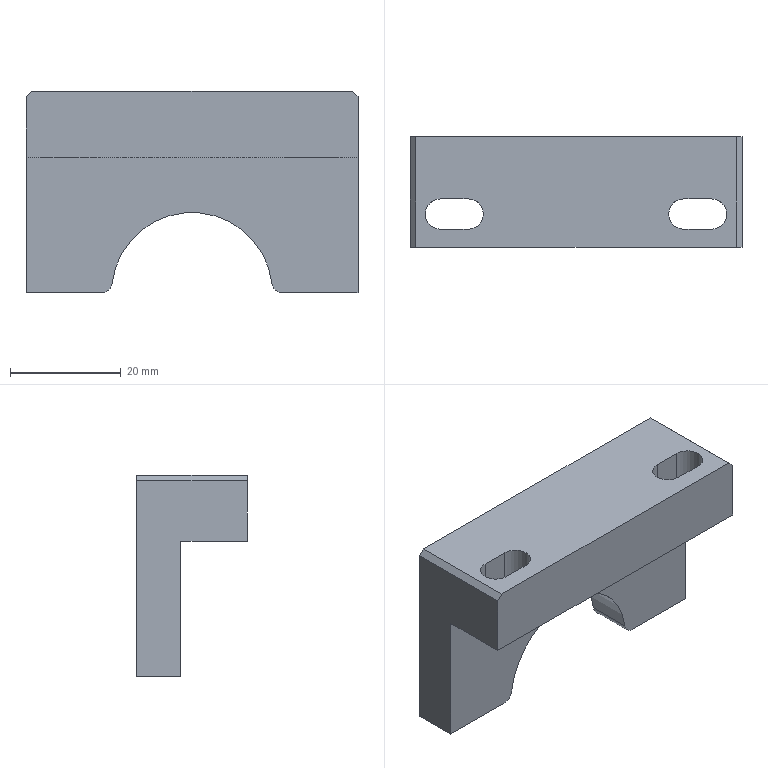Part | NX | 1 solid | 26 faces | box 60 x 20 x 36.5 mm | volume 22060 mm3 | plane 15 | cylinder 9 | cone 2 | commonest cylinder face diameters 5.5 x4 3.3 x2 4 x2 29.1 x1
STEP:
#1=CARTESIAN_POINT('',(24.5,3.75,6.25));
#2=VERTEX_POINT('',#1);
#3=CARTESIAN_POINT('',(24.5,3.75,18.25));
#4=VERTEX_POINT('',#3);
#5=CARTESIAN_POINT('',(24.5,3.75,-18.25));
#6=DIRECTION('',(0.,0.,1.));
#7=VECTOR('',#6,1000.);
#8=LINE('',#5,#7);
#9=EDGE_CURVE('',#2,#4,#8,.T.);
#10=ORIENTED_EDGE('',*,*,#9,.T.);
#11=CARTESIAN_POINT('',(19.5,3.75,18.25));
#12=VERTEX_POINT('',#11);
#13=CARTESIAN_POINT('',(24.5,3.75,18.25));
#14=DIRECTION('',(-1.,0.,0.));
#15=VECTOR('',#14,1000.);
#16=LINE('',#13,#15);
#17=EDGE_CURVE('',#4,#12,#16,.T.);
#18=ORIENTED_EDGE('',*,*,#17,.T.);
#19=CARTESIAN_POINT('',(19.5,3.75,6.25));
#20=VERTEX_POINT('',#19);
#21=CARTESIAN_POINT('',(19.5,3.75,-18.25));
#22=DIRECTION('',(0.,0.,1.));
#23=VECTOR('',#22,1000.);
#24=LINE('',#21,#23);
#25=EDGE_CURVE('',#20,#12,#24,.T.);
#26=ORIENTED_EDGE('',*,*,#25,.F.);
#27=CARTESIAN_POINT('',(-30.,3.75,6.25));
#28=DIRECTION('',(-1.,0.,0.));
#29=VECTOR('',#28,1000.);
#30=LINE('',#27,#29);
#31=EDGE_CURVE('',#2,#20,#30,.T.);
#32=ORIENTED_EDGE('',*,*,#31,.F.);
#33=EDGE_LOOP('',(#10,#18,#26,#32));
#34=FACE_BOUND('',#33,.T.);
#35=CARTESIAN_POINT('',(24.5,3.75,-18.25));
#36=DIRECTION('',(0.,1.,0.));
#37=DIRECTION('',(-1.,0.,0.));
#38=AXIS2_PLACEMENT_3D('',#35,#36,#37);
#39=PLANE('',#38);
#40=ADVANCED_FACE('',(#34),#39,.F.);
#41=ORIENTED_EDGE('',*,*,#25,.T.);
#42=CARTESIAN_POINT('',(19.5,-1.75,18.25));
#43=VERTEX_POINT('',#42);
#44=CARTESIAN_POINT('',(19.5,1.,18.25));
#45=DIRECTION('',(0.,0.,1.));
#46=DIRECTION('',(1.,0.,0.));
#47=AXIS2_PLACEMENT_3D('',#44,#45,#46);
#48=CIRCLE('',#47,2.75);
#49=EDGE_CURVE('',#12,#43,#48,.T.);
#50=ORIENTED_EDGE('',*,*,#49,.T.);
#51=CARTESIAN_POINT('',(19.5,-1.75,6.25));
#52=VERTEX_POINT('',#51);
#53=CARTESIAN_POINT('',(19.5,-1.75,-18.25));
#54=DIRECTION('',(0.,0.,1.));
#55=VECTOR('',#54,1000.);
#56=LINE('',#53,#55);
#57=EDGE_CURVE('',#52,#43,#56,.T.);
#58=ORIENTED_EDGE('',*,*,#57,.F.);
#59=CARTESIAN_POINT('',(19.5,1.,6.25));
#60=DIRECTION('',(0.,0.,1.));
#61=DIRECTION('',(1.,0.,0.));
#62=AXIS2_PLACEMENT_3D('',#59,#60,#61);
#63=CIRCLE('',#62,2.75);
#64=EDGE_CURVE('',#20,#52,#63,.T.);
#65=ORIENTED_EDGE('',*,*,#64,.F.);
#66=EDGE_LOOP('',(#41,#50,#58,#65));
#67=FACE_BOUND('',#66,.T.);
#68=CARTESIAN_POINT('',(19.5,1.,-18.25));
#69=DIRECTION('',(0.,0.,1.));
#70=DIRECTION('',(1.,0.,0.));
#71=AXIS2_PLACEMENT_3D('',#68,#69,#70);
#72=CYLINDRICAL_SURFACE('',#71,2.75);
#73=ADVANCED_FACE('',(#67),#72,.F.);
#74=ORIENTED_EDGE('',*,*,#57,.T.);
#75=CARTESIAN_POINT('',(24.5,-1.75,18.25));
#76=VERTEX_POINT('',#75);
#77=CARTESIAN_POINT('',(24.5,-1.75,18.25));
#78=DIRECTION('',(1.,0.,0.));
#79=VECTOR('',#78,1000.);
#80=LINE('',#77,#79);
#81=EDGE_CURVE('',#43,#76,#80,.T.);
#82=ORIENTED_EDGE('',*,*,#81,.T.);
#83=CARTESIAN_POINT('',(24.5,-1.75,6.25));
#84=VERTEX_POINT('',#83);
#85=CARTESIAN_POINT('',(24.5,-1.75,-18.25));
#86=DIRECTION('',(0.,0.,1.));
#87=VECTOR('',#86,1000.);
#88=LINE('',#85,#87);
#89=EDGE_CURVE('',#84,#76,#88,.T.);
#90=ORIENTED_EDGE('',*,*,#89,.F.);
#91=CARTESIAN_POINT('',(-30.,-1.75,6.25));
#92=DIRECTION('',(1.,0.,0.));
#93=VECTOR('',#92,1000.);
#94=LINE('',#91,#93);
#95=EDGE_CURVE('',#52,#84,#94,.T.);
#96=ORIENTED_EDGE('',*,*,#95,.F.);
#97=EDGE_LOOP('',(#74,#82,#90,#96));
#98=FACE_BOUND('',#97,.T.);
#99=CARTESIAN_POINT('',(24.5,-1.75,-18.25));
#100=DIRECTION('',(0.,-1.,0.));
#101=DIRECTION('',(1.,0.,0.));
#102=AXIS2_PLACEMENT_3D('',#99,#100,#101);
#103=PLANE('',#102);
#104=ADVANCED_FACE('',(#98),#103,.F.);
#105=CARTESIAN_POINT('',(-19.5,3.75,6.25));
#106=VERTEX_POINT('',#105);
#107=CARTESIAN_POINT('',(-19.5,3.75,18.25));
#108=VERTEX_POINT('',#107);
#109=CARTESIAN_POINT('',(-19.5,3.75,-18.25));
#110=DIRECTION('',(0.,0.,1.));
#111=VECTOR('',#110,1000.);
#112=LINE('',#109,#111);
#113=EDGE_CURVE('',#106,#108,#112,.T.);
#114=ORIENTED_EDGE('',*,*,#113,.T.);
#115=CARTESIAN_POINT('',(-24.5,3.75,18.25));
#116=VERTEX_POINT('',#115);
#117=CARTESIAN_POINT('',(24.5,3.75,18.25));
#118=DIRECTION('',(-1.,0.,0.));
#119=VECTOR('',#118,1000.);
#120=LINE('',#117,#119);
#121=EDGE_CURVE('',#108,#116,#120,.T.);
#122=ORIENTED_EDGE('',*,*,#121,.T.);
#123=CARTESIAN_POINT('',(-24.5,3.75,6.25));
#124=VERTEX_POINT('',#123);
#125=CARTESIAN_POINT('',(-24.5,3.75,-18.25));
#126=DIRECTION('',(0.,0.,1.));
#127=VECTOR('',#126,1000.);
#128=LINE('',#125,#127);
#129=EDGE_CURVE('',#124,#116,#128,.T.);
#130=ORIENTED_EDGE('',*,*,#129,.F.);
#131=CARTESIAN_POINT('',(-30.,3.75,6.25));
#132=DIRECTION('',(-1.,0.,0.));
#133=VECTOR('',#132,1000.);
#134=LINE('',#131,#133);
#135=EDGE_CURVE('',#106,#124,#134,.T.);
#136=ORIENTED_EDGE('',*,*,#135,.F.);
#137=EDGE_LOOP('',(#114,#122,#130,#136));
#138=FACE_BOUND('',#137,.T.);
#139=CARTESIAN_POINT('',(24.5,3.75,-18.25));
#140=DIRECTION('',(0.,1.,0.));
#141=DIRECTION('',(-1.,0.,0.));
#142=AXIS2_PLACEMENT_3D('',#139,#140,#141);
#143=PLANE('',#142);
#144=ADVANCED_FACE('',(#138),#143,.F.);
#145=ORIENTED_EDGE('',*,*,#129,.T.);
#146=CARTESIAN_POINT('',(-24.5,-1.75,18.25));
#147=VERTEX_POINT('',#146);
#148=CARTESIAN_POINT('',(-24.5,1.,18.25));
#149=DIRECTION('',(0.,0.,1.));
#150=DIRECTION('',(1.,0.,0.));
#151=AXIS2_PLACEMENT_3D('',#148,#149,#150);
#152=CIRCLE('',#151,2.75);
#153=EDGE_CURVE('',#116,#147,#152,.T.);
#154=ORIENTED_EDGE('',*,*,#153,.T.);
#155=CARTESIAN_POINT('',(-24.5,-1.75,6.25));
#156=VERTEX_POINT('',#155);
#157=CARTESIAN_POINT('',(-24.5,-1.75,-18.25));
#158=DIRECTION('',(0.,0.,1.));
#159=VECTOR('',#158,1000.);
#160=LINE('',#157,#159);
#161=EDGE_CURVE('',#156,#147,#160,.T.);
#162=ORIENTED_EDGE('',*,*,#161,.F.);
#163=CARTESIAN_POINT('',(-24.5,1.,6.25));
#164=DIRECTION('',(0.,0.,1.));
#165=DIRECTION('',(1.,0.,0.));
#166=AXIS2_PLACEMENT_3D('',#163,#164,#165);
#167=CIRCLE('',#166,2.75);
#168=EDGE_CURVE('',#124,#156,#167,.T.);
#169=ORIENTED_EDGE('',*,*,#168,.F.);
#170=EDGE_LOOP('',(#145,#154,#162,#169));
#171=FACE_BOUND('',#170,.T.);
#172=CARTESIAN_POINT('',(-24.5,1.,-18.25));
#173=DIRECTION('',(0.,0.,1.));
#174=DIRECTION('',(1.,0.,0.));
#175=AXIS2_PLACEMENT_3D('',#172,#173,#174);
#176=CYLINDRICAL_SURFACE('',#175,2.75);
#177=ADVANCED_FACE('',(#171),#176,.F.);
#178=ORIENTED_EDGE('',*,*,#161,.T.);
#179=CARTESIAN_POINT('',(-19.5,-1.75,18.25));
#180=VERTEX_POINT('',#179);
#181=CARTESIAN_POINT('',(24.5,-1.75,18.25));
#182=DIRECTION('',(1.,0.,0.));
#183=VECTOR('',#182,1000.);
#184=LINE('',#181,#183);
#185=EDGE_CURVE('',#147,#180,#184,.T.);
#186=ORIENTED_EDGE('',*,*,#185,.T.);
#187=CARTESIAN_POINT('',(-19.5,-1.75,6.25));
#188=VERTEX_POINT('',#187);
#189=CARTESIAN_POINT('',(-19.5,-1.75,-18.25));
#190=DIRECTION('',(0.,0.,1.));
#191=VECTOR('',#190,1000.);
#192=LINE('',#189,#191);
#193=EDGE_CURVE('',#188,#180,#192,.T.);
#194=ORIENTED_EDGE('',*,*,#193,.F.);
#195=CARTESIAN_POINT('',(-30.,-1.75,6.25));
#196=DIRECTION('',(1.,0.,0.));
#197=VECTOR('',#196,1000.);
#198=LINE('',#195,#197);
#199=EDGE_CURVE('',#156,#188,#198,.T.);
#200=ORIENTED_EDGE('',*,*,#199,.F.);
#201=EDGE_LOOP('',(#178,#186,#194,#200));
#202=FACE_BOUND('',#201,.T.);
#203=CARTESIAN_POINT('',(24.5,-1.75,-18.25));
#204=DIRECTION('',(0.,-1.,0.));
#205=DIRECTION('',(1.,0.,0.));
#206=AXIS2_PLACEMENT_3D('',#203,#204,#205);
#207=PLANE('',#206);
#208=ADVANCED_FACE('',(#202),#207,.F.);
#209=CARTESIAN_POINT('',(14.443,7.,-16.492));
#210=VERTEX_POINT('',#209);
#211=CARTESIAN_POINT('',(16.429,7.,-18.25));
#212=VERTEX_POINT('',#211);
#213=CARTESIAN_POINT('',(16.429,7.,-16.25));
#214=DIRECTION('',(0.,-1.,0.));
#215=DIRECTION('',(0.,0.,1.));
#216=AXIS2_PLACEMENT_3D('',#213,#214,#215);
#217=CIRCLE('',#216,2.);
#218=EDGE_CURVE('',#210,#212,#217,.T.);
#219=ORIENTED_EDGE('',*,*,#218,.T.);
#220=CARTESIAN_POINT('',(30.,7.,-18.25));
#221=VERTEX_POINT('',#220);
#222=CARTESIAN_POINT('',(-30.,7.,-18.25));
#223=DIRECTION('',(1.,0.,0.));
#224=VECTOR('',#223,1000.);
#225=LINE('',#222,#224);
#226=EDGE_CURVE('',#212,#221,#225,.T.);
#227=ORIENTED_EDGE('',*,*,#226,.T.);
#228=CARTESIAN_POINT('',(30.,7.,6.25));
#229=VERTEX_POINT('',#228);
#230=CARTESIAN_POINT('',(30.,7.,-18.25));
#231=DIRECTION('',(0.,0.,1.));
#232=VECTOR('',#231,1000.);
#233=LINE('',#230,#232);
#234=EDGE_CURVE('',#221,#229,#233,.T.);
#235=ORIENTED_EDGE('',*,*,#234,.T.);
#236=CARTESIAN_POINT('',(-30.,7.,6.25));
#237=VERTEX_POINT('',#236);
#238=CARTESIAN_POINT('',(-30.,7.,6.25));
#239=DIRECTION('',(1.,0.,0.));
#240=VECTOR('',#239,1000.);
#241=LINE('',#238,#240);
#242=EDGE_CURVE('',#237,#229,#241,.T.);
#243=ORIENTED_EDGE('',*,*,#242,.F.);
#244=CARTESIAN_POINT('',(-30.,7.,-18.25));
#245=VERTEX_POINT('',#244);
#246=CARTESIAN_POINT('',(-30.,7.,-18.25));
#247=DIRECTION('',(0.,0.,1.));
#248=VECTOR('',#247,1000.);
#249=LINE('',#246,#248);
#250=EDGE_CURVE('',#245,#237,#249,.T.);
#251=ORIENTED_EDGE('',*,*,#250,.F.);
#252=CARTESIAN_POINT('',(-16.429,7.,-18.25));
#253=VERTEX_POINT('',#252);
#254=CARTESIAN_POINT('',(-30.,7.,-18.25));
#255=DIRECTION('',(1.,0.,0.));
#256=VECTOR('',#255,1000.);
#257=LINE('',#254,#256);
#258=EDGE_CURVE('',#245,#253,#257,.T.);
#259=ORIENTED_EDGE('',*,*,#258,.T.);
#260=CARTESIAN_POINT('',(-14.443,7.,-16.492));
#261=VERTEX_POINT('',#260);
#262=CARTESIAN_POINT('',(-16.429,7.,-16.25));
#263=DIRECTION('',(0.,-1.,0.));
#264=DIRECTION('',(0.,0.,1.));
#265=AXIS2_PLACEMENT_3D('',#262,#263,#264);
#266=CIRCLE('',#265,2.);
#267=EDGE_CURVE('',#253,#261,#266,.T.);
#268=ORIENTED_EDGE('',*,*,#267,.T.);
#269=CARTESIAN_POINT('',(0.,7.,-18.25));
#270=DIRECTION('',(0.,-1.,0.));
#271=DIRECTION('',(0.,0.,1.));
#272=AXIS2_PLACEMENT_3D('',#269,#270,#271);
#273=CIRCLE('',#272,14.55);
#274=EDGE_CURVE('',#210,#261,#273,.T.);
#275=ORIENTED_EDGE('',*,*,#274,.F.);
#276=EDGE_LOOP('',(#219,#227,#235,#243,#251,#259,#268,#275));
#277=FACE_BOUND('',#276,.T.);
#278=CARTESIAN_POINT('',(-30.,7.,-18.25));
#279=DIRECTION('',(0.,1.,0.));
#280=DIRECTION('',(0.,0.,1.));
#281=AXIS2_PLACEMENT_3D('',#278,#279,#280);
#282=PLANE('',#281);
#283=ADVANCED_FACE('',(#277),#282,.F.);
#284=CARTESIAN_POINT('',(30.,-5.,6.25));
#285=VERTEX_POINT('',#284);
#286=CARTESIAN_POINT('',(30.,-5.,6.25));
#287=DIRECTION('',(0.,-1.,0.));
#288=VECTOR('',#287,1000.);
#289=LINE('',#286,#288);
#290=EDGE_CURVE('',#229,#285,#289,.T.);
#291=ORIENTED_EDGE('',*,*,#290,.T.);
#292=CARTESIAN_POINT('',(-30.,-5.,6.25));
#293=VERTEX_POINT('',#292);
#294=CARTESIAN_POINT('',(-30.,-5.,6.25));
#295=DIRECTION('',(1.,0.,0.));
#296=VECTOR('',#295,1000.);
#297=LINE('',#294,#296);
#298=EDGE_CURVE('',#293,#285,#297,.T.);
#299=ORIENTED_EDGE('',*,*,#298,.F.);
#300=CARTESIAN_POINT('',(-30.,-5.,6.25));
#301=DIRECTION('',(0.,-1.,0.));
#302=VECTOR('',#301,1000.);
#303=LINE('',#300,#302);
#304=EDGE_CURVE('',#237,#293,#303,.T.);
#305=ORIENTED_EDGE('',*,*,#304,.F.);
#306=ORIENTED_EDGE('',*,*,#242,.T.);
#307=EDGE_LOOP('',(#291,#299,#305,#306));
#308=FACE_BOUND('',#307,.T.);
#309=ORIENTED_EDGE('',*,*,#199,.T.);
#310=CARTESIAN_POINT('',(-19.5,1.,6.25));
#311=DIRECTION('',(0.,0.,1.));
#312=DIRECTION('',(1.,0.,0.));
#313=AXIS2_PLACEMENT_3D('',#310,#311,#312);
#314=CIRCLE('',#313,2.75);
#315=EDGE_CURVE('',#188,#106,#314,.T.);
#316=ORIENTED_EDGE('',*,*,#315,.T.);
#317=ORIENTED_EDGE('',*,*,#135,.T.);
#318=ORIENTED_EDGE('',*,*,#168,.T.);
#319=EDGE_LOOP('',(#309,#316,#317,#318));
#320=FACE_BOUND('',#319,.T.);
#321=ORIENTED_EDGE('',*,*,#95,.T.);
#322=CARTESIAN_POINT('',(24.5,1.,6.25));
#323=DIRECTION('',(0.,0.,1.));
#324=DIRECTION('',(1.,0.,0.));
#325=AXIS2_PLACEMENT_3D('',#322,#323,#324);
#326=CIRCLE('',#325,2.75);
#327=EDGE_CURVE('',#84,#2,#326,.T.);
#328=ORIENTED_EDGE('',*,*,#327,.T.);
#329=ORIENTED_EDGE('',*,*,#31,.T.);
#330=ORIENTED_EDGE('',*,*,#64,.T.);
#331=EDGE_LOOP('',(#321,#328,#329,#330));
#332=FACE_BOUND('',#331,.T.);
#333=CARTESIAN_POINT('',(-30.,-5.,6.25));
#334=DIRECTION('',(0.,0.,1.));
#335=DIRECTION('',(1.,0.,0.));
#336=AXIS2_PLACEMENT_3D('',#333,#334,#335);
#337=PLANE('',#336);
#338=ADVANCED_FACE('',(#308,#320,#332),#337,.F.);
#339=ORIENTED_EDGE('',*,*,#267,.F.);
#340=CARTESIAN_POINT('',(-16.429,15.,-18.25));
#341=VERTEX_POINT('',#340);
#342=CARTESIAN_POINT('',(-16.429,15.,-18.25));
#343=DIRECTION('',(0.,1.,0.));
#344=VECTOR('',#343,1000.);
#345=LINE('',#342,#344);
#346=EDGE_CURVE('',#341,#253,#345,.F.);
#347=ORIENTED_EDGE('',*,*,#346,.F.);
#348=CARTESIAN_POINT('',(-14.443,15.,-16.492));
#349=VERTEX_POINT('',#348);
#350=CARTESIAN_POINT('',(-16.429,15.,-16.25));
#351=DIRECTION('',(0.,1.,0.));
#352=DIRECTION('',(0.,0.,-1.));
#353=AXIS2_PLACEMENT_3D('',#350,#351,#352);
#354=CIRCLE('',#353,2.);
#355=EDGE_CURVE('',#349,#341,#354,.T.);
#356=ORIENTED_EDGE('',*,*,#355,.F.);
#357=CARTESIAN_POINT('',(-14.443,7.,-16.492));
#358=DIRECTION('',(0.,-1.,0.));
#359=VECTOR('',#358,1000.);
#360=LINE('',#357,#359);
#361=EDGE_CURVE('',#261,#349,#360,.F.);
#362=ORIENTED_EDGE('',*,*,#361,.F.);
#363=EDGE_LOOP('',(#339,#347,#356,#362));
#364=FACE_BOUND('',#363,.T.);
#365=CARTESIAN_POINT('',(-16.429,15.,-16.25));
#366=DIRECTION('',(0.,-1.,0.));
#367=DIRECTION('',(0.,0.,-1.));
#368=AXIS2_PLACEMENT_3D('',#365,#366,#367);
#369=CYLINDRICAL_SURFACE('',#368,2.);
#370=ADVANCED_FACE('',(#364),#369,.T.);
#371=ORIENTED_EDGE('',*,*,#218,.F.);
#372=CARTESIAN_POINT('',(14.443,15.,-16.492));
#373=VERTEX_POINT('',#372);
#374=CARTESIAN_POINT('',(14.443,15.,-16.492));
#375=DIRECTION('',(0.,-1.,0.));
#376=VECTOR('',#375,1000.);
#377=LINE('',#374,#376);
#378=EDGE_CURVE('',#373,#210,#377,.T.);
#379=ORIENTED_EDGE('',*,*,#378,.F.);
#380=CARTESIAN_POINT('',(16.429,15.,-18.25));
#381=VERTEX_POINT('',#380);
#382=CARTESIAN_POINT('',(16.429,15.,-16.25));
#383=DIRECTION('',(0.,1.,0.));
#384=DIRECTION('',(0.,0.,-1.));
#385=AXIS2_PLACEMENT_3D('',#382,#383,#384);
#386=CIRCLE('',#385,2.);
#387=EDGE_CURVE('',#381,#373,#386,.T.);
#388=ORIENTED_EDGE('',*,*,#387,.F.);
#389=CARTESIAN_POINT('',(16.429,15.,-18.25));
#390=DIRECTION('',(0.,1.,0.));
#391=VECTOR('',#390,1000.);
#392=LINE('',#389,#391);
#393=EDGE_CURVE('',#212,#381,#392,.T.);
#394=ORIENTED_EDGE('',*,*,#393,.F.);
#395=EDGE_LOOP('',(#371,#379,#388,#394));
#396=FACE_BOUND('',#395,.T.);
#397=CARTESIAN_POINT('',(16.429,15.,-16.25));
#398=DIRECTION('',(0.,-1.,0.));
#399=DIRECTION('',(0.,0.,-1.));
#400=AXIS2_PLACEMENT_3D('',#397,#398,#399);
#401=CYLINDRICAL_SURFACE('',#400,2.);
#402=ADVANCED_FACE('',(#396),#401,.T.);
#403=CARTESIAN_POINT('',(29.,15.,18.25));
#404=VERTEX_POINT('',#403);
#405=CARTESIAN_POINT('',(30.,15.,17.25));
#406=VERTEX_POINT('',#405);
#407=CARTESIAN_POINT('',(30.,15.,17.25));
#408=DIRECTION('',(0.7071,0.,-0.7071));
#409=VECTOR('',#408,1000.);
#410=LINE('',#407,#409);
#411=EDGE_CURVE('',#404,#406,#410,.T.);
#412=ORIENTED_EDGE('',*,*,#411,.F.);
#413=CARTESIAN_POINT('',(29.,-5.,18.25));
#414=VERTEX_POINT('',#413);
#415=CARTESIAN_POINT('',(29.,15.,18.25));
#416=DIRECTION('',(0.,1.,0.));
#417=VECTOR('',#416,1000.);
#418=LINE('',#415,#417);
#419=EDGE_CURVE('',#414,#404,#418,.T.);
#420=ORIENTED_EDGE('',*,*,#419,.F.);
#421=CARTESIAN_POINT('',(30.,-5.,17.25));
#422=VERTEX_POINT('',#421);
#423=CARTESIAN_POINT('',(23.625,-5.,23.625));
#424=DIRECTION('',(-0.7071,0.,0.7071));
#425=VECTOR('',#424,1000.);
#426=LINE('',#423,#425);
#427=EDGE_CURVE('',#422,#414,#426,.T.);
#428=ORIENTED_EDGE('',*,*,#427,.F.);
#429=CARTESIAN_POINT('',(30.,15.,17.25));
#430=DIRECTION('',(0.,-1.,0.));
#431=VECTOR('',#430,1000.);
#432=LINE('',#429,#431);
#433=EDGE_CURVE('',#406,#422,#432,.T.);
#434=ORIENTED_EDGE('',*,*,#433,.F.);
#435=EDGE_LOOP('',(#412,#420,#428,#434));
#436=FACE_BOUND('',#435,.T.);
#437=CARTESIAN_POINT('',(30.,15.,17.25));
#438=DIRECTION('',(-0.7071,0.,-0.7071));
#439=DIRECTION('',(0.,-1.,0.));
#440=AXIS2_PLACEMENT_3D('',#437,#438,#439);
#441=PLANE('',#440);
#442=ADVANCED_FACE('',(#436),#441,.F.);
#443=CARTESIAN_POINT('',(-30.,15.,17.25));
#444=VERTEX_POINT('',#443);
#445=CARTESIAN_POINT('',(-29.,15.,18.25));
#446=VERTEX_POINT('',#445);
#447=CARTESIAN_POINT('',(-29.,15.,18.25));
#448=DIRECTION('',(0.7071,0.,0.7071));
#449=VECTOR('',#448,1000.);
#450=LINE('',#447,#449);
#451=EDGE_CURVE('',#444,#446,#450,.T.);
#452=ORIENTED_EDGE('',*,*,#451,.F.);
#453=CARTESIAN_POINT('',(-30.,-5.,17.25));
#454=VERTEX_POINT('',#453);
#455=CARTESIAN_POINT('',(-30.,15.,17.25));
#456=DIRECTION('',(0.,1.,0.));
#457=VECTOR('',#456,1000.);
#458=LINE('',#455,#457);
#459=EDGE_CURVE('',#454,#444,#458,.T.);
#460=ORIENTED_EDGE('',*,*,#459,.F.);
#461=CARTESIAN_POINT('',(-29.,-5.,18.25));
#462=VERTEX_POINT('',#461);
#463=CARTESIAN_POINT('',(-23.625,-5.,23.625));
#464=DIRECTION('',(-0.7071,0.,-0.7071));
#465=VECTOR('',#464,1000.);
#466=LINE('',#463,#465);
#467=EDGE_CURVE('',#462,#454,#466,.T.);
#468=ORIENTED_EDGE('',*,*,#467,.F.);
#469=CARTESIAN_POINT('',(-29.,15.,18.25));
#470=DIRECTION('',(0.,-1.,0.));
#471=VECTOR('',#470,1000.);
#472=LINE('',#469,#471);
#473=EDGE_CURVE('',#446,#462,#472,.T.);
#474=ORIENTED_EDGE('',*,*,#473,.F.);
#475=EDGE_LOOP('',(#452,#460,#468,#474));
#476=FACE_BOUND('',#475,.T.);
#477=CARTESIAN_POINT('',(-29.,15.,18.25));
#478=DIRECTION('',(0.7071,0.,-0.7071));
#479=DIRECTION('',(0.,-1.,0.));
#480=AXIS2_PLACEMENT_3D('',#477,#478,#479);
#481=PLANE('',#480);
#482=ADVANCED_FACE('',(#476),#481,.F.);
#483=ORIENTED_EDGE('',*,*,#378,.T.);
#484=ORIENTED_EDGE('',*,*,#274,.T.);
#485=ORIENTED_EDGE('',*,*,#361,.T.);
#486=CARTESIAN_POINT('',(0.,15.,-18.25));
#487=DIRECTION('',(0.,-1.,0.));
#488=DIRECTION('',(0.,0.,-1.));
#489=AXIS2_PLACEMENT_3D('',#486,#487,#488);
#490=CIRCLE('',#489,14.55);
#491=EDGE_CURVE('',#373,#349,#490,.T.);
#492=ORIENTED_EDGE('',*,*,#491,.F.);
#493=EDGE_LOOP('',(#483,#484,#485,#492));
#494=FACE_BOUND('',#493,.T.);
#495=CARTESIAN_POINT('',(0.,15.,-18.25));
#496=DIRECTION('',(0.,-1.,0.));
#497=DIRECTION('',(0.,0.,-1.));
#498=AXIS2_PLACEMENT_3D('',#495,#496,#497);
#499=CYLINDRICAL_SURFACE('',#498,14.55);
#500=ADVANCED_FACE('',(#494),#499,.F.);
#501=ORIENTED_EDGE('',*,*,#298,.T.);
#502=CARTESIAN_POINT('',(30.,-5.,-18.25));
#503=DIRECTION('',(0.,0.,1.));
#504=VECTOR('',#503,1000.);
#505=LINE('',#502,#504);
#506=EDGE_CURVE('',#285,#422,#505,.T.);
#507=ORIENTED_EDGE('',*,*,#506,.T.);
#508=ORIENTED_EDGE('',*,*,#427,.T.);
#509=CARTESIAN_POINT('',(30.,-5.,18.25));
#510=DIRECTION('',(-1.,0.,0.));
#511=VECTOR('',#510,1000.);
#512=LINE('',#509,#511);
#513=EDGE_CURVE('',#414,#462,#512,.T.);
#514=ORIENTED_EDGE('',*,*,#513,.T.);
#515=ORIENTED_EDGE('',*,*,#467,.T.);
#516=CARTESIAN_POINT('',(-30.,-5.,18.25));
#517=DIRECTION('',(0.,0.,-1.));
#518=VECTOR('',#517,1000.);
#519=LINE('',#516,#518);
#520=EDGE_CURVE('',#454,#293,#519,.T.);
#521=ORIENTED_EDGE('',*,*,#520,.T.);
#522=EDGE_LOOP('',(#501,#507,#508,#514,#515,#521));
#523=FACE_BOUND('',#522,.T.);
#524=CARTESIAN_POINT('',(0.,-5.,0.));
#525=DIRECTION('',(0.,-1.,0.));
#526=DIRECTION('',(0.,0.,-1.));
#527=AXIS2_PLACEMENT_3D('',#524,#525,#526);
#528=PLANE('',#527);
#529=ADVANCED_FACE('',(#523),#528,.T.);
#530=CARTESIAN_POINT('',(30.,15.,-18.25));
#531=VERTEX_POINT('',#530);
#532=CARTESIAN_POINT('',(-30.,15.,-18.25));
#533=DIRECTION('',(1.,0.,0.));
#534=VECTOR('',#533,1000.);
#535=LINE('',#532,#534);
#536=EDGE_CURVE('',#381,#531,#535,.T.);
#537=ORIENTED_EDGE('',*,*,#536,.F.);
#538=ORIENTED_EDGE('',*,*,#387,.T.);
#539=ORIENTED_EDGE('',*,*,#491,.T.);
#540=ORIENTED_EDGE('',*,*,#355,.T.);
#541=CARTESIAN_POINT('',(-30.,15.,-18.25));
#542=VERTEX_POINT('',#541);
#543=CARTESIAN_POINT('',(-30.,15.,-18.25));
#544=DIRECTION('',(1.,0.,0.));
#545=VECTOR('',#544,1000.);
#546=LINE('',#543,#545);
#547=EDGE_CURVE('',#542,#341,#546,.T.);
#548=ORIENTED_EDGE('',*,*,#547,.F.);
#549=CARTESIAN_POINT('',(-30.,15.,18.25));
#550=DIRECTION('',(0.,0.,-1.));
#551=VECTOR('',#550,1000.);
#552=LINE('',#549,#551);
#553=EDGE_CURVE('',#444,#542,#552,.T.);
#554=ORIENTED_EDGE('',*,*,#553,.F.);
#555=ORIENTED_EDGE('',*,*,#451,.T.);
#556=CARTESIAN_POINT('',(30.,15.,18.25));
#557=DIRECTION('',(-1.,0.,0.));
#558=VECTOR('',#557,1000.);
#559=LINE('',#556,#558);
#560=EDGE_CURVE('',#404,#446,#559,.T.);
#561=ORIENTED_EDGE('',*,*,#560,.F.);
#562=ORIENTED_EDGE('',*,*,#411,.T.);
#563=CARTESIAN_POINT('',(30.,15.,-18.25));
#564=DIRECTION('',(0.,0.,1.));
#565=VECTOR('',#564,1000.);
#566=LINE('',#563,#565);
#567=EDGE_CURVE('',#531,#406,#566,.T.);
#568=ORIENTED_EDGE('',*,*,#567,.F.);
#569=EDGE_LOOP('',(#537,#538,#539,#540,#548,#554,#555,#561,#562,#568));
#570=FACE_BOUND('',#569,.T.);
#571=CARTESIAN_POINT('',(0.,15.,0.));
#572=DIRECTION('',(0.,-1.,0.));
#573=DIRECTION('',(0.,0.,-1.));
#574=AXIS2_PLACEMENT_3D('',#571,#572,#573);
#575=PLANE('',#574);
#576=ADVANCED_FACE('',(#570),#575,.F.);
#577=ORIENTED_EDGE('',*,*,#304,.T.);
#578=ORIENTED_EDGE('',*,*,#520,.F.);
#579=ORIENTED_EDGE('',*,*,#459,.T.);
#580=ORIENTED_EDGE('',*,*,#553,.T.);
#581=CARTESIAN_POINT('',(-30.,15.,-18.25));
#582=DIRECTION('',(0.,-1.,0.));
#583=VECTOR('',#582,1000.);
#584=LINE('',#581,#583);
#585=EDGE_CURVE('',#542,#245,#584,.T.);
#586=ORIENTED_EDGE('',*,*,#585,.T.);
#587=ORIENTED_EDGE('',*,*,#250,.T.);
#588=EDGE_LOOP('',(#577,#578,#579,#580,#586,#587));
#589=FACE_BOUND('',#588,.T.);
#590=CARTESIAN_POINT('',(-30.,15.,18.25));
#591=DIRECTION('',(-1.,0.,0.));
#592=DIRECTION('',(0.,0.,1.));
#593=AXIS2_PLACEMENT_3D('',#590,#591,#592);
#594=PLANE('',#593);
#595=ADVANCED_FACE('',(#589),#594,.T.);
#596=CARTESIAN_POINT('',(-26.65,11.,-18.25));
#597=VERTEX_POINT('',#596);
#598=CARTESIAN_POINT('',(-25.,11.,-18.25));
#599=DIRECTION('',(0.,0.,-1.));
#600=DIRECTION('',(-1.,0.,0.));
#601=AXIS2_PLACEMENT_3D('',#598,#599,#600);
#602=CIRCLE('',#601,1.65);
#603=EDGE_CURVE('',#597,#597,#602,.T.);
#604=ORIENTED_EDGE('',*,*,#603,.F.);
#605=EDGE_LOOP('',(#604));
#606=FACE_BOUND('',#605,.T.);
#607=ORIENTED_EDGE('',*,*,#258,.F.);
#608=ORIENTED_EDGE('',*,*,#585,.F.);
#609=ORIENTED_EDGE('',*,*,#547,.T.);
#610=ORIENTED_EDGE('',*,*,#346,.T.);
#611=EDGE_LOOP('',(#607,#608,#609,#610));
#612=FACE_BOUND('',#611,.T.);
#613=CARTESIAN_POINT('',(-30.,15.,-18.25));
#614=DIRECTION('',(0.,0.,-1.));
#615=DIRECTION('',(-1.,0.,0.));
#616=AXIS2_PLACEMENT_3D('',#613,#614,#615);
#617=PLANE('',#616);
#618=ADVANCED_FACE('',(#606,#612),#617,.T.);
#619=ORIENTED_EDGE('',*,*,#290,.F.);
#620=ORIENTED_EDGE('',*,*,#234,.F.);
#621=CARTESIAN_POINT('',(30.,15.,-18.25));
#622=DIRECTION('',(0.,-1.,0.));
#623=VECTOR('',#622,1000.);
#624=LINE('',#621,#623);
#625=EDGE_CURVE('',#531,#221,#624,.T.);
#626=ORIENTED_EDGE('',*,*,#625,.F.);
#627=ORIENTED_EDGE('',*,*,#567,.T.);
#628=ORIENTED_EDGE('',*,*,#433,.T.);
#629=ORIENTED_EDGE('',*,*,#506,.F.);
#630=EDGE_LOOP('',(#619,#620,#626,#627,#628,#629));
#631=FACE_BOUND('',#630,.T.);
#632=CARTESIAN_POINT('',(30.,15.,-18.25));
#633=DIRECTION('',(1.,0.,0.));
#634=DIRECTION('',(0.,0.,-1.));
#635=AXIS2_PLACEMENT_3D('',#632,#633,#634);
#636=PLANE('',#635);
#637=ADVANCED_FACE('',(#631),#636,.T.);
#638=ORIENTED_EDGE('',*,*,#560,.T.);
#639=ORIENTED_EDGE('',*,*,#473,.T.);
#640=ORIENTED_EDGE('',*,*,#513,.F.);
#641=ORIENTED_EDGE('',*,*,#419,.T.);
#642=EDGE_LOOP('',(#638,#639,#640,#641));
#643=FACE_BOUND('',#642,.T.);
#644=CARTESIAN_POINT('',(-19.5,1.,18.25));
#645=DIRECTION('',(0.,0.,1.));
#646=DIRECTION('',(1.,0.,0.));
#647=AXIS2_PLACEMENT_3D('',#644,#645,#646);
#648=CIRCLE('',#647,2.75);
#649=EDGE_CURVE('',#180,#108,#648,.T.);
#650=ORIENTED_EDGE('',*,*,#649,.F.);
#651=ORIENTED_EDGE('',*,*,#185,.F.);
#652=ORIENTED_EDGE('',*,*,#153,.F.);
#653=ORIENTED_EDGE('',*,*,#121,.F.);
#654=EDGE_LOOP('',(#650,#651,#652,#653));
#655=FACE_BOUND('',#654,.T.);
#656=CARTESIAN_POINT('',(24.5,1.,18.25));
#657=DIRECTION('',(0.,0.,1.));
#658=DIRECTION('',(1.,0.,0.));
#659=AXIS2_PLACEMENT_3D('',#656,#657,#658);
#660=CIRCLE('',#659,2.75);
#661=EDGE_CURVE('',#76,#4,#660,.T.);
#662=ORIENTED_EDGE('',*,*,#661,.F.);
#663=ORIENTED_EDGE('',*,*,#81,.F.);
#664=ORIENTED_EDGE('',*,*,#49,.F.);
#665=ORIENTED_EDGE('',*,*,#17,.F.);
#666=EDGE_LOOP('',(#662,#663,#664,#665));
#667=FACE_BOUND('',#666,.T.);
#668=CARTESIAN_POINT('',(30.,15.,18.25));
#669=DIRECTION('',(0.,0.,1.));
#670=DIRECTION('',(1.,0.,0.));
#671=AXIS2_PLACEMENT_3D('',#668,#669,#670);
#672=PLANE('',#671);
#673=ADVANCED_FACE('',(#643,#655,#667),#672,.T.);
#674=CARTESIAN_POINT('',(23.35,11.,-18.25));
#675=VERTEX_POINT('',#674);
#676=CARTESIAN_POINT('',(25.,11.,-18.25));
#677=DIRECTION('',(0.,0.,-1.));
#678=DIRECTION('',(-1.,0.,0.));
#679=AXIS2_PLACEMENT_3D('',#676,#677,#678);
#680=CIRCLE('',#679,1.65);
#681=EDGE_CURVE('',#675,#675,#680,.T.);
#682=ORIENTED_EDGE('',*,*,#681,.F.);
#683=EDGE_LOOP('',(#682));
#684=FACE_BOUND('',#683,.T.);
#685=ORIENTED_EDGE('',*,*,#226,.F.);
#686=ORIENTED_EDGE('',*,*,#393,.T.);
#687=ORIENTED_EDGE('',*,*,#536,.T.);
#688=ORIENTED_EDGE('',*,*,#625,.T.);
#689=EDGE_LOOP('',(#685,#686,#687,#688));
#690=FACE_BOUND('',#689,.T.);
#691=CARTESIAN_POINT('',(-30.,15.,-18.25));
#692=DIRECTION('',(0.,0.,-1.));
#693=DIRECTION('',(-1.,0.,0.));
#694=AXIS2_PLACEMENT_3D('',#691,#692,#693);
#695=PLANE('',#694);
#696=ADVANCED_FACE('',(#684,#690),#695,.T.);
#697=CARTESIAN_POINT('',(25.,11.,-7.159));
#698=VERTEX_POINT('',#697);
#699=VERTEX_LOOP('',#698);
#700=FACE_BOUND('',#699,.T.);
#701=CARTESIAN_POINT('',(23.35,11.,-8.15));
#702=VERTEX_POINT('',#701);
#703=CARTESIAN_POINT('',(25.,11.,-8.15));
#704=DIRECTION('',(0.,0.,-1.));
#705=DIRECTION('',(-1.,0.,0.));
#706=AXIS2_PLACEMENT_3D('',#703,#704,#705);
#707=CIRCLE('',#706,1.65);
#708=EDGE_CURVE('',#702,#702,#707,.T.);
#709=ORIENTED_EDGE('',*,*,#708,.T.);
#710=EDGE_LOOP('',(#709));
#711=FACE_BOUND('',#710,.T.);
#712=CARTESIAN_POINT('',(25.,11.,-8.15));
#713=DIRECTION('',(0.,0.,-1.));
#714=DIRECTION('',(-1.,0.,0.));
#715=AXIS2_PLACEMENT_3D('',#712,#713,#714);
#716=CONICAL_SURFACE('',#715,1.65,1.03);
#717=ADVANCED_FACE('',(#700,#711),#716,.F.);
#718=ORIENTED_EDGE('',*,*,#681,.T.);
#719=EDGE_LOOP('',(#718));
#720=FACE_BOUND('',#719,.T.);
#721=ORIENTED_EDGE('',*,*,#708,.F.);
#722=EDGE_LOOP('',(#721));
#723=FACE_BOUND('',#722,.T.);
#724=CARTESIAN_POINT('',(25.,11.,-18.25));
#725=DIRECTION('',(0.,0.,-1.));
#726=DIRECTION('',(-1.,0.,0.));
#727=AXIS2_PLACEMENT_3D('',#724,#725,#726);
#728=CYLINDRICAL_SURFACE('',#727,1.65);
#729=ADVANCED_FACE('',(#720,#723),#728,.F.);
#730=CARTESIAN_POINT('',(-25.,11.,-7.159));
#731=VERTEX_POINT('',#730);
#732=VERTEX_LOOP('',#731);
#733=FACE_BOUND('',#732,.T.);
#734=CARTESIAN_POINT('',(-26.65,11.,-8.15));
#735=VERTEX_POINT('',#734);
#736=CARTESIAN_POINT('',(-25.,11.,-8.15));
#737=DIRECTION('',(0.,0.,-1.));
#738=DIRECTION('',(-1.,0.,0.));
#739=AXIS2_PLACEMENT_3D('',#736,#737,#738);
#740=CIRCLE('',#739,1.65);
#741=EDGE_CURVE('',#735,#735,#740,.T.);
#742=ORIENTED_EDGE('',*,*,#741,.T.);
#743=EDGE_LOOP('',(#742));
#744=FACE_BOUND('',#743,.T.);
#745=CARTESIAN_POINT('',(-25.,11.,-8.15));
#746=DIRECTION('',(0.,0.,-1.));
#747=DIRECTION('',(-1.,0.,0.));
#748=AXIS2_PLACEMENT_3D('',#745,#746,#747);
#749=CONICAL_SURFACE('',#748,1.65,1.03);
#750=ADVANCED_FACE('',(#733,#744),#749,.F.);
#751=ORIENTED_EDGE('',*,*,#603,.T.);
#752=EDGE_LOOP('',(#751));
#753=FACE_BOUND('',#752,.T.);
#754=ORIENTED_EDGE('',*,*,#741,.F.);
#755=EDGE_LOOP('',(#754));
#756=FACE_BOUND('',#755,.T.);
#757=CARTESIAN_POINT('',(-25.,11.,-18.25));
#758=DIRECTION('',(0.,0.,-1.));
#759=DIRECTION('',(-1.,0.,0.));
#760=AXIS2_PLACEMENT_3D('',#757,#758,#759);
#761=CYLINDRICAL_SURFACE('',#760,1.65);
#762=ADVANCED_FACE('',(#753,#756),#761,.F.);
#763=ORIENTED_EDGE('',*,*,#315,.F.);
#764=ORIENTED_EDGE('',*,*,#193,.T.);
#765=ORIENTED_EDGE('',*,*,#649,.T.);
#766=ORIENTED_EDGE('',*,*,#113,.F.);
#767=EDGE_LOOP('',(#763,#764,#765,#766));
#768=FACE_BOUND('',#767,.T.);
#769=CARTESIAN_POINT('',(-19.5,1.,-18.25));
#770=DIRECTION('',(0.,0.,1.));
#771=DIRECTION('',(1.,0.,0.));
#772=AXIS2_PLACEMENT_3D('',#769,#770,#771);
#773=CYLINDRICAL_SURFACE('',#772,2.75);
#774=ADVANCED_FACE('',(#768),#773,.F.);
#775=ORIENTED_EDGE('',*,*,#327,.F.);
#776=ORIENTED_EDGE('',*,*,#89,.T.);
#777=ORIENTED_EDGE('',*,*,#661,.T.);
#778=ORIENTED_EDGE('',*,*,#9,.F.);
#779=EDGE_LOOP('',(#775,#776,#777,#778));
#780=FACE_BOUND('',#779,.T.);
#781=CARTESIAN_POINT('',(24.5,1.,-18.25));
#782=DIRECTION('',(0.,0.,1.));
#783=DIRECTION('',(1.,0.,0.));
#784=AXIS2_PLACEMENT_3D('',#781,#782,#783);
#785=CYLINDRICAL_SURFACE('',#784,2.75);
#786=ADVANCED_FACE('',(#780),#785,.F.);
#787=CLOSED_SHELL('',(#40,#73,#104,#144,#177,#208,#283,#338,#370,#402,#442,#482,#500,#529,#576,#595,#618,#637,#673,#696,#717,#729,#750,#762,#774,#786));
#788=MANIFOLD_SOLID_BREP('',#787);
#789=(LENGTH_UNIT()NAMED_UNIT(*)SI_UNIT(.MILLI.,.METRE.));
#790=UNCERTAINTY_MEASURE_WITH_UNIT(LENGTH_MEASURE(0.00001),#789,'','');
#791=(NAMED_UNIT(*)PLANE_ANGLE_UNIT()SI_UNIT($,.RADIAN.));
#792=(NAMED_UNIT(*)SI_UNIT($,.STERADIAN.)SOLID_ANGLE_UNIT());
#793=(GEOMETRIC_REPRESENTATION_CONTEXT(3)GLOBAL_UNCERTAINTY_ASSIGNED_CONTEXT((#790))GLOBAL_UNIT_ASSIGNED_CONTEXT((#789,#791,#792))REPRESENTATION_CONTEXT('',''));
#794=ADVANCED_BREP_SHAPE_REPRESENTATION('',(#788),#793);